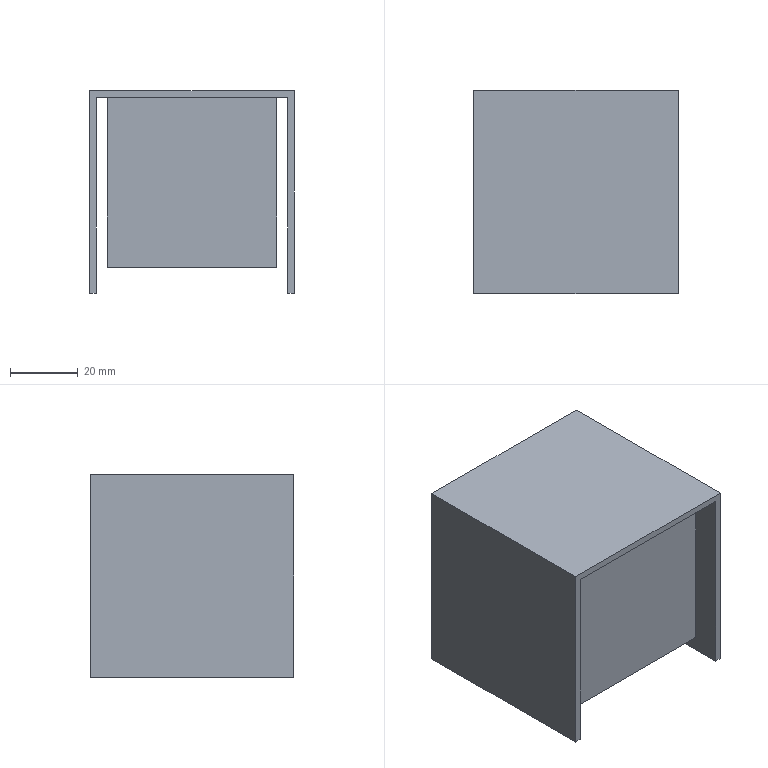Part | SolidWorks | features ICE 5, BaseBody 1 | 1 solid | 15 faces | box 60.365 x 60 x 59.674 mm | volume 146086 mm3 | plane 15
STEP:
#1=CARTESIAN_POINT('',(58.25,-37.247,42.006));
#2=VERTEX_POINT('',#1);
#3=CARTESIAN_POINT('',(1.886,-37.247,42.006));
#4=VERTEX_POINT('',#3);
#5=CARTESIAN_POINT('',(1.886,-37.247,42.006));
#6=DIRECTION('',(-1.,0.,0.));
#7=VECTOR('',#6,1000.);
#8=LINE('',#5,#7);
#9=EDGE_CURVE('',#2,#4,#8,.T.);
#10=ORIENTED_EDGE('',*,*,#9,.T.);
#11=CARTESIAN_POINT('',(1.886,22.753,42.006));
#12=VERTEX_POINT('',#11);
#13=CARTESIAN_POINT('',(1.886,22.753,42.006));
#14=DIRECTION('',(0.,-1.,0.));
#15=VECTOR('',#14,1000.);
#16=LINE('',#13,#15);
#17=EDGE_CURVE('',#12,#4,#16,.T.);
#18=ORIENTED_EDGE('',*,*,#17,.F.);
#19=CARTESIAN_POINT('',(58.25,22.753,42.006));
#20=VERTEX_POINT('',#19);
#21=CARTESIAN_POINT('',(1.886,22.753,42.006));
#22=DIRECTION('',(-1.,0.,0.));
#23=VECTOR('',#22,1000.);
#24=LINE('',#21,#23);
#25=EDGE_CURVE('',#20,#12,#24,.T.);
#26=ORIENTED_EDGE('',*,*,#25,.F.);
#27=CARTESIAN_POINT('',(58.25,22.753,42.006));
#28=DIRECTION('',(0.,-1.,0.));
#29=VECTOR('',#28,1000.);
#30=LINE('',#27,#29);
#31=EDGE_CURVE('',#20,#2,#30,.T.);
#32=ORIENTED_EDGE('',*,*,#31,.T.);
#33=EDGE_LOOP('',(#10,#18,#26,#32));
#34=FACE_OUTER_BOUND('',#33,.T.);
#35=CARTESIAN_POINT('',(55.068,17.753,42.006));
#36=VERTEX_POINT('',#35);
#37=CARTESIAN_POINT('',(55.068,-32.247,42.006));
#38=VERTEX_POINT('',#37);
#39=CARTESIAN_POINT('',(55.068,-32.247,42.006));
#40=DIRECTION('',(0.,-1.,0.));
#41=VECTOR('',#40,1000.);
#42=LINE('',#39,#41);
#43=EDGE_CURVE('',#36,#38,#42,.T.);
#44=ORIENTED_EDGE('',*,*,#43,.F.);
#45=CARTESIAN_POINT('',(5.068,17.753,42.006));
#46=VERTEX_POINT('',#45);
#47=CARTESIAN_POINT('',(55.068,17.753,42.006));
#48=DIRECTION('',(1.,0.,0.));
#49=VECTOR('',#48,1000.);
#50=LINE('',#47,#49);
#51=EDGE_CURVE('',#46,#36,#50,.T.);
#52=ORIENTED_EDGE('',*,*,#51,.F.);
#53=CARTESIAN_POINT('',(5.068,-32.247,42.006));
#54=VERTEX_POINT('',#53);
#55=CARTESIAN_POINT('',(5.068,17.753,42.006));
#56=DIRECTION('',(0.,1.,0.));
#57=VECTOR('',#56,1000.);
#58=LINE('',#55,#57);
#59=EDGE_CURVE('',#54,#46,#58,.T.);
#60=ORIENTED_EDGE('',*,*,#59,.F.);
#61=CARTESIAN_POINT('',(5.068,-32.247,42.006));
#62=DIRECTION('',(-1.,0.,0.));
#63=VECTOR('',#62,1000.);
#64=LINE('',#61,#63);
#65=EDGE_CURVE('',#38,#54,#64,.T.);
#66=ORIENTED_EDGE('',*,*,#65,.F.);
#67=EDGE_LOOP('',(#44,#52,#60,#66));
#68=FACE_BOUND('',#67,.T.);
#69=CARTESIAN_POINT('',(1.886,22.753,42.006));
#70=DIRECTION('',(0.,0.,1.));
#71=DIRECTION('',(0.,-1.,0.));
#72=AXIS2_PLACEMENT_3D('',#69,#70,#71);
#73=PLANE('',#72);
#74=ADVANCED_FACE('',(#34,#68),#73,.F.);
#75=CARTESIAN_POINT('',(1.886,22.753,-15.668));
#76=VERTEX_POINT('',#75);
#77=CARTESIAN_POINT('',(-0.1143,22.753,-15.668));
#78=VERTEX_POINT('',#77);
#79=CARTESIAN_POINT('',(60.,22.753,-15.668));
#80=DIRECTION('',(-1.,0.,0.));
#81=VECTOR('',#80,1000.);
#82=LINE('',#79,#81);
#83=EDGE_CURVE('',#76,#78,#82,.T.);
#84=ORIENTED_EDGE('',*,*,#83,.F.);
#85=CARTESIAN_POINT('',(1.886,-37.247,-15.668));
#86=VERTEX_POINT('',#85);
#87=CARTESIAN_POINT('',(1.886,-37.247,-15.668));
#88=DIRECTION('',(0.,-1.,0.));
#89=VECTOR('',#88,1000.);
#90=LINE('',#87,#89);
#91=EDGE_CURVE('',#76,#86,#90,.T.);
#92=ORIENTED_EDGE('',*,*,#91,.T.);
#93=CARTESIAN_POINT('',(-0.1143,-37.247,-15.668));
#94=VERTEX_POINT('',#93);
#95=CARTESIAN_POINT('',(60.,-37.247,-15.668));
#96=DIRECTION('',(-1.,0.,0.));
#97=VECTOR('',#96,1000.);
#98=LINE('',#95,#97);
#99=EDGE_CURVE('',#86,#94,#98,.T.);
#100=ORIENTED_EDGE('',*,*,#99,.T.);
#101=CARTESIAN_POINT('',(-0.1143,22.753,-15.668));
#102=DIRECTION('',(0.,-1.,0.));
#103=VECTOR('',#102,1000.);
#104=LINE('',#101,#103);
#105=EDGE_CURVE('',#78,#94,#104,.T.);
#106=ORIENTED_EDGE('',*,*,#105,.F.);
#107=EDGE_LOOP('',(#84,#92,#100,#106));
#108=FACE_OUTER_BOUND('',#107,.T.);
#109=CARTESIAN_POINT('',(60.,-37.247,-15.668));
#110=DIRECTION('',(0.,0.,1.));
#111=DIRECTION('',(1.,0.,0.));
#112=AXIS2_PLACEMENT_3D('',#109,#110,#111);
#113=PLANE('',#112);
#114=ADVANCED_FACE('',(#108),#113,.F.);
#115=CARTESIAN_POINT('',(60.25,-37.247,-15.668));
#116=VERTEX_POINT('',#115);
#117=CARTESIAN_POINT('',(60.25,-37.247,44.006));
#118=VERTEX_POINT('',#117);
#119=CARTESIAN_POINT('',(60.25,-37.247,-15.668));
#120=DIRECTION('',(0.,0.,1.));
#121=VECTOR('',#120,1000.);
#122=LINE('',#119,#121);
#123=EDGE_CURVE('',#116,#118,#122,.T.);
#124=ORIENTED_EDGE('',*,*,#123,.T.);
#125=CARTESIAN_POINT('',(-0.1143,-37.247,44.006));
#126=VERTEX_POINT('',#125);
#127=CARTESIAN_POINT('',(-0.1143,-37.247,44.006));
#128=DIRECTION('',(-1.,0.,0.));
#129=VECTOR('',#128,1000.);
#130=LINE('',#127,#129);
#131=EDGE_CURVE('',#118,#126,#130,.T.);
#132=ORIENTED_EDGE('',*,*,#131,.T.);
#133=CARTESIAN_POINT('',(-0.1143,-37.247,44.332));
#134=DIRECTION('',(0.,0.,-1.));
#135=VECTOR('',#134,1000.);
#136=LINE('',#133,#135);
#137=EDGE_CURVE('',#126,#94,#136,.T.);
#138=ORIENTED_EDGE('',*,*,#137,.T.);
#139=ORIENTED_EDGE('',*,*,#99,.F.);
#140=CARTESIAN_POINT('',(1.886,-37.247,42.006));
#141=DIRECTION('',(0.,0.,-1.));
#142=VECTOR('',#141,1000.);
#143=LINE('',#140,#142);
#144=EDGE_CURVE('',#4,#86,#143,.T.);
#145=ORIENTED_EDGE('',*,*,#144,.F.);
#146=ORIENTED_EDGE('',*,*,#9,.F.);
#147=CARTESIAN_POINT('',(58.25,-37.247,-15.668));
#148=VERTEX_POINT('',#147);
#149=CARTESIAN_POINT('',(58.25,-37.247,42.006));
#150=DIRECTION('',(0.,0.,1.));
#151=VECTOR('',#150,1000.);
#152=LINE('',#149,#151);
#153=EDGE_CURVE('',#148,#2,#152,.T.);
#154=ORIENTED_EDGE('',*,*,#153,.F.);
#155=CARTESIAN_POINT('',(60.,-37.247,-15.668));
#156=DIRECTION('',(-1.,0.,0.));
#157=VECTOR('',#156,1000.);
#158=LINE('',#155,#157);
#159=EDGE_CURVE('',#116,#148,#158,.T.);
#160=ORIENTED_EDGE('',*,*,#159,.F.);
#161=EDGE_LOOP('',(#124,#132,#138,#139,#145,#146,#154,#160));
#162=FACE_OUTER_BOUND('',#161,.T.);
#163=CARTESIAN_POINT('',(60.,-37.247,44.332));
#164=DIRECTION('',(0.,1.,0.));
#165=DIRECTION('',(0.,0.,1.));
#166=AXIS2_PLACEMENT_3D('',#163,#164,#165);
#167=PLANE('',#166);
#168=ADVANCED_FACE('',(#162),#167,.F.);
#169=ORIENTED_EDGE('',*,*,#159,.T.);
#170=CARTESIAN_POINT('',(58.25,22.753,-15.668));
#171=VERTEX_POINT('',#170);
#172=CARTESIAN_POINT('',(58.25,-37.247,-15.668));
#173=DIRECTION('',(0.,1.,0.));
#174=VECTOR('',#173,1000.);
#175=LINE('',#172,#174);
#176=EDGE_CURVE('',#148,#171,#175,.T.);
#177=ORIENTED_EDGE('',*,*,#176,.T.);
#178=CARTESIAN_POINT('',(60.25,22.753,-15.668));
#179=VERTEX_POINT('',#178);
#180=CARTESIAN_POINT('',(60.,22.753,-15.668));
#181=DIRECTION('',(-1.,0.,0.));
#182=VECTOR('',#181,1000.);
#183=LINE('',#180,#182);
#184=EDGE_CURVE('',#179,#171,#183,.T.);
#185=ORIENTED_EDGE('',*,*,#184,.F.);
#186=CARTESIAN_POINT('',(60.25,22.753,-15.668));
#187=DIRECTION('',(0.,-1.,0.));
#188=VECTOR('',#187,1000.);
#189=LINE('',#186,#188);
#190=EDGE_CURVE('',#179,#116,#189,.T.);
#191=ORIENTED_EDGE('',*,*,#190,.T.);
#192=EDGE_LOOP('',(#169,#177,#185,#191));
#193=FACE_OUTER_BOUND('',#192,.T.);
#194=CARTESIAN_POINT('',(60.,-37.247,-15.668));
#195=DIRECTION('',(0.,0.,1.));
#196=DIRECTION('',(1.,0.,0.));
#197=AXIS2_PLACEMENT_3D('',#194,#195,#196);
#198=PLANE('',#197);
#199=ADVANCED_FACE('',(#193),#198,.F.);
#200=CARTESIAN_POINT('',(-0.1143,22.753,44.006));
#201=VERTEX_POINT('',#200);
#202=CARTESIAN_POINT('',(-0.1143,22.753,44.332));
#203=DIRECTION('',(0.,0.,-1.));
#204=VECTOR('',#203,1000.);
#205=LINE('',#202,#204);
#206=EDGE_CURVE('',#201,#78,#205,.T.);
#207=ORIENTED_EDGE('',*,*,#206,.F.);
#208=CARTESIAN_POINT('',(60.25,22.753,44.006));
#209=VERTEX_POINT('',#208);
#210=CARTESIAN_POINT('',(-0.1143,22.753,44.006));
#211=DIRECTION('',(-1.,0.,0.));
#212=VECTOR('',#211,1000.);
#213=LINE('',#210,#212);
#214=EDGE_CURVE('',#209,#201,#213,.T.);
#215=ORIENTED_EDGE('',*,*,#214,.F.);
#216=CARTESIAN_POINT('',(60.25,22.753,-15.668));
#217=DIRECTION('',(0.,0.,1.));
#218=VECTOR('',#217,1000.);
#219=LINE('',#216,#218);
#220=EDGE_CURVE('',#179,#209,#219,.T.);
#221=ORIENTED_EDGE('',*,*,#220,.F.);
#222=ORIENTED_EDGE('',*,*,#184,.T.);
#223=CARTESIAN_POINT('',(58.25,22.753,44.332));
#224=DIRECTION('',(0.,0.,1.));
#225=VECTOR('',#224,1000.);
#226=LINE('',#223,#225);
#227=EDGE_CURVE('',#171,#20,#226,.T.);
#228=ORIENTED_EDGE('',*,*,#227,.T.);
#229=ORIENTED_EDGE('',*,*,#25,.T.);
#230=CARTESIAN_POINT('',(1.886,22.753,42.006));
#231=DIRECTION('',(0.,0.,-1.));
#232=VECTOR('',#231,1000.);
#233=LINE('',#230,#232);
#234=EDGE_CURVE('',#12,#76,#233,.T.);
#235=ORIENTED_EDGE('',*,*,#234,.T.);
#236=ORIENTED_EDGE('',*,*,#83,.T.);
#237=EDGE_LOOP('',(#207,#215,#221,#222,#228,#229,#235,#236));
#238=FACE_OUTER_BOUND('',#237,.T.);
#239=CARTESIAN_POINT('',(60.,22.753,44.332));
#240=DIRECTION('',(0.,-1.,0.));
#241=DIRECTION('',(0.,0.,-1.));
#242=AXIS2_PLACEMENT_3D('',#239,#240,#241);
#243=PLANE('',#242);
#244=ADVANCED_FACE('',(#238),#243,.F.);
#245=ORIENTED_EDGE('',*,*,#234,.F.);
#246=ORIENTED_EDGE('',*,*,#17,.T.);
#247=ORIENTED_EDGE('',*,*,#144,.T.);
#248=ORIENTED_EDGE('',*,*,#91,.F.);
#249=EDGE_LOOP('',(#245,#246,#247,#248));
#250=FACE_OUTER_BOUND('',#249,.T.);
#251=CARTESIAN_POINT('',(1.886,22.753,42.006));
#252=DIRECTION('',(-1.,0.,0.));
#253=DIRECTION('',(0.,0.,1.));
#254=AXIS2_PLACEMENT_3D('',#251,#252,#253);
#255=PLANE('',#254);
#256=ADVANCED_FACE('',(#250),#255,.F.);
#257=ORIENTED_EDGE('',*,*,#153,.T.);
#258=ORIENTED_EDGE('',*,*,#31,.F.);
#259=ORIENTED_EDGE('',*,*,#227,.F.);
#260=ORIENTED_EDGE('',*,*,#176,.F.);
#261=EDGE_LOOP('',(#257,#258,#259,#260));
#262=FACE_OUTER_BOUND('',#261,.T.);
#263=CARTESIAN_POINT('',(58.25,22.753,42.006));
#264=DIRECTION('',(1.,0.,0.));
#265=DIRECTION('',(0.,0.,-1.));
#266=AXIS2_PLACEMENT_3D('',#263,#264,#265);
#267=PLANE('',#266);
#268=ADVANCED_FACE('',(#262),#267,.F.);
#269=ORIENTED_EDGE('',*,*,#43,.T.);
#270=CARTESIAN_POINT('',(55.068,-32.247,-7.994));
#271=VERTEX_POINT('',#270);
#272=CARTESIAN_POINT('',(55.068,-32.247,-7.994));
#273=DIRECTION('',(0.,0.,1.));
#274=VECTOR('',#273,1000.);
#275=LINE('',#272,#274);
#276=EDGE_CURVE('',#271,#38,#275,.T.);
#277=ORIENTED_EDGE('',*,*,#276,.F.);
#278=CARTESIAN_POINT('',(55.068,17.753,-7.994));
#279=VERTEX_POINT('',#278);
#280=CARTESIAN_POINT('',(55.068,-32.247,-7.994));
#281=DIRECTION('',(0.,-1.,0.));
#282=VECTOR('',#281,1000.);
#283=LINE('',#280,#282);
#284=EDGE_CURVE('',#279,#271,#283,.T.);
#285=ORIENTED_EDGE('',*,*,#284,.F.);
#286=CARTESIAN_POINT('',(55.068,17.753,-7.994));
#287=DIRECTION('',(0.,0.,1.));
#288=VECTOR('',#287,1000.);
#289=LINE('',#286,#288);
#290=EDGE_CURVE('',#279,#36,#289,.T.);
#291=ORIENTED_EDGE('',*,*,#290,.T.);
#292=EDGE_LOOP('',(#269,#277,#285,#291));
#293=FACE_OUTER_BOUND('',#292,.T.);
#294=CARTESIAN_POINT('',(55.068,-32.247,-7.994));
#295=DIRECTION('',(-1.,0.,0.));
#296=DIRECTION('',(0.,0.,1.));
#297=AXIS2_PLACEMENT_3D('',#294,#295,#296);
#298=PLANE('',#297);
#299=ADVANCED_FACE('',(#293),#298,.F.);
#300=ORIENTED_EDGE('',*,*,#65,.T.);
#301=CARTESIAN_POINT('',(5.068,-32.247,-7.994));
#302=VERTEX_POINT('',#301);
#303=CARTESIAN_POINT('',(5.068,-32.247,-7.994));
#304=DIRECTION('',(0.,0.,1.));
#305=VECTOR('',#304,1000.);
#306=LINE('',#303,#305);
#307=EDGE_CURVE('',#302,#54,#306,.T.);
#308=ORIENTED_EDGE('',*,*,#307,.F.);
#309=CARTESIAN_POINT('',(5.068,-32.247,-7.994));
#310=DIRECTION('',(-1.,0.,0.));
#311=VECTOR('',#310,1000.);
#312=LINE('',#309,#311);
#313=EDGE_CURVE('',#271,#302,#312,.T.);
#314=ORIENTED_EDGE('',*,*,#313,.F.);
#315=ORIENTED_EDGE('',*,*,#276,.T.);
#316=EDGE_LOOP('',(#300,#308,#314,#315));
#317=FACE_OUTER_BOUND('',#316,.T.);
#318=CARTESIAN_POINT('',(5.068,-32.247,-7.994));
#319=DIRECTION('',(0.,1.,0.));
#320=DIRECTION('',(0.,0.,1.));
#321=AXIS2_PLACEMENT_3D('',#318,#319,#320);
#322=PLANE('',#321);
#323=ADVANCED_FACE('',(#317),#322,.F.);
#324=ORIENTED_EDGE('',*,*,#59,.T.);
#325=CARTESIAN_POINT('',(5.068,17.753,-7.994));
#326=VERTEX_POINT('',#325);
#327=CARTESIAN_POINT('',(5.068,17.753,-7.994));
#328=DIRECTION('',(0.,0.,1.));
#329=VECTOR('',#328,1000.);
#330=LINE('',#327,#329);
#331=EDGE_CURVE('',#326,#46,#330,.T.);
#332=ORIENTED_EDGE('',*,*,#331,.F.);
#333=CARTESIAN_POINT('',(5.068,17.753,-7.994));
#334=DIRECTION('',(0.,1.,0.));
#335=VECTOR('',#334,1000.);
#336=LINE('',#333,#335);
#337=EDGE_CURVE('',#302,#326,#336,.T.);
#338=ORIENTED_EDGE('',*,*,#337,.F.);
#339=ORIENTED_EDGE('',*,*,#307,.T.);
#340=EDGE_LOOP('',(#324,#332,#338,#339));
#341=FACE_OUTER_BOUND('',#340,.T.);
#342=CARTESIAN_POINT('',(5.068,17.753,-7.994));
#343=DIRECTION('',(1.,0.,0.));
#344=DIRECTION('',(0.,0.,-1.));
#345=AXIS2_PLACEMENT_3D('',#342,#343,#344);
#346=PLANE('',#345);
#347=ADVANCED_FACE('',(#341),#346,.F.);
#348=ORIENTED_EDGE('',*,*,#51,.T.);
#349=ORIENTED_EDGE('',*,*,#290,.F.);
#350=CARTESIAN_POINT('',(55.068,17.753,-7.994));
#351=DIRECTION('',(1.,0.,0.));
#352=VECTOR('',#351,1000.);
#353=LINE('',#350,#352);
#354=EDGE_CURVE('',#326,#279,#353,.T.);
#355=ORIENTED_EDGE('',*,*,#354,.F.);
#356=ORIENTED_EDGE('',*,*,#331,.T.);
#357=EDGE_LOOP('',(#348,#349,#355,#356));
#358=FACE_OUTER_BOUND('',#357,.T.);
#359=CARTESIAN_POINT('',(55.068,17.753,-7.994));
#360=DIRECTION('',(0.,-1.,0.));
#361=DIRECTION('',(0.,0.,-1.));
#362=AXIS2_PLACEMENT_3D('',#359,#360,#361);
#363=PLANE('',#362);
#364=ADVANCED_FACE('',(#358),#363,.F.);
#365=ORIENTED_EDGE('',*,*,#284,.T.);
#366=ORIENTED_EDGE('',*,*,#313,.T.);
#367=ORIENTED_EDGE('',*,*,#337,.T.);
#368=ORIENTED_EDGE('',*,*,#354,.T.);
#369=EDGE_LOOP('',(#365,#366,#367,#368));
#370=FACE_OUTER_BOUND('',#369,.T.);
#371=CARTESIAN_POINT('',(0.,0.,-7.994));
#372=DIRECTION('',(0.,0.,1.));
#373=DIRECTION('',(0.,-1.,0.));
#374=AXIS2_PLACEMENT_3D('',#371,#372,#373);
#375=PLANE('',#374);
#376=ADVANCED_FACE('',(#370),#375,.F.);
#377=CARTESIAN_POINT('',(-0.1143,-37.247,44.006));
#378=DIRECTION('',(0.,1.,0.));
#379=VECTOR('',#378,1000.);
#380=LINE('',#377,#379);
#381=EDGE_CURVE('',#126,#201,#380,.T.);
#382=ORIENTED_EDGE('',*,*,#381,.T.);
#383=ORIENTED_EDGE('',*,*,#206,.T.);
#384=ORIENTED_EDGE('',*,*,#105,.T.);
#385=ORIENTED_EDGE('',*,*,#137,.F.);
#386=EDGE_LOOP('',(#382,#383,#384,#385));
#387=FACE_OUTER_BOUND('',#386,.T.);
#388=CARTESIAN_POINT('',(-0.1143,22.753,44.332));
#389=DIRECTION('',(-1.,0.,0.));
#390=DIRECTION('',(0.,0.,1.));
#391=AXIS2_PLACEMENT_3D('',#388,#389,#390);
#392=PLANE('',#391);
#393=ADVANCED_FACE('',(#387),#392,.T.);
#394=CARTESIAN_POINT('',(60.25,-37.247,44.006));
#395=DIRECTION('',(0.,1.,0.));
#396=VECTOR('',#395,1000.);
#397=LINE('',#394,#396);
#398=EDGE_CURVE('',#118,#209,#397,.T.);
#399=ORIENTED_EDGE('',*,*,#398,.F.);
#400=ORIENTED_EDGE('',*,*,#123,.F.);
#401=ORIENTED_EDGE('',*,*,#190,.F.);
#402=ORIENTED_EDGE('',*,*,#220,.T.);
#403=EDGE_LOOP('',(#399,#400,#401,#402));
#404=FACE_OUTER_BOUND('',#403,.T.);
#405=CARTESIAN_POINT('',(60.25,22.753,-15.668));
#406=DIRECTION('',(1.,0.,0.));
#407=DIRECTION('',(0.,0.,-1.));
#408=AXIS2_PLACEMENT_3D('',#405,#406,#407);
#409=PLANE('',#408);
#410=ADVANCED_FACE('',(#404),#409,.T.);
#411=ORIENTED_EDGE('',*,*,#214,.T.);
#412=ORIENTED_EDGE('',*,*,#381,.F.);
#413=ORIENTED_EDGE('',*,*,#131,.F.);
#414=ORIENTED_EDGE('',*,*,#398,.T.);
#415=EDGE_LOOP('',(#411,#412,#413,#414));
#416=FACE_OUTER_BOUND('',#415,.T.);
#417=CARTESIAN_POINT('',(-0.1143,-37.247,44.006));
#418=DIRECTION('',(0.,0.,-1.));
#419=DIRECTION('',(0.,1.,0.));
#420=AXIS2_PLACEMENT_3D('',#417,#418,#419);
#421=PLANE('',#420);
#422=ADVANCED_FACE('',(#416),#421,.F.);
#423=CLOSED_SHELL('',(#74,#114,#168,#199,#244,#256,#268,#299,#323,#347,#364,#376,#393,#410,#422));
#424=MANIFOLD_SOLID_BREP('',#423);
#425=CARTESIAN_POINT('',(0.,0.,0.));
#426=DIRECTION('',(0.,0.,1.));
#427=DIRECTION('',(1.,0.,0.));
#428=AXIS2_PLACEMENT_3D('',#425,#426,#427);
#429=(LENGTH_UNIT()NAMED_UNIT(*)SI_UNIT(.MILLI.,.METRE.));
#430=UNCERTAINTY_MEASURE_WITH_UNIT(LENGTH_MEASURE(0.00001),#429,'','');
#431=(NAMED_UNIT(*)PLANE_ANGLE_UNIT()SI_UNIT($,.RADIAN.));
#432=(NAMED_UNIT(*)SI_UNIT($,.STERADIAN.)SOLID_ANGLE_UNIT());
#433=(GEOMETRIC_REPRESENTATION_CONTEXT(3)GLOBAL_UNCERTAINTY_ASSIGNED_CONTEXT((#430))GLOBAL_UNIT_ASSIGNED_CONTEXT((#429,#431,#432))REPRESENTATION_CONTEXT('',''));
#434=ADVANCED_BREP_SHAPE_REPRESENTATION('',(#424,#428),#433);